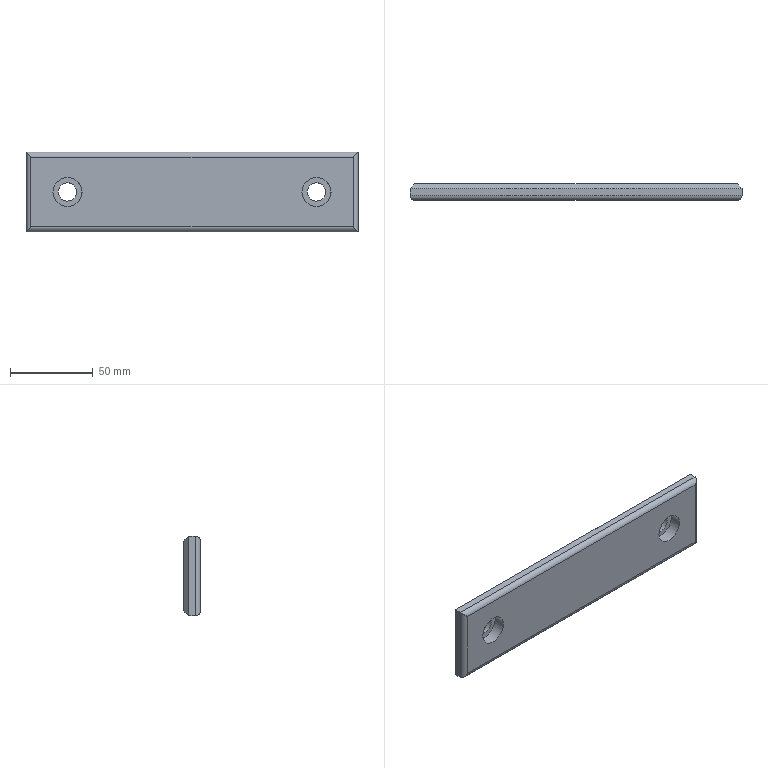Part | NX | features solid 2 | 1 solid | 20 faces | box 200 x 10 x 48 mm | volume 88919 mm3 | plane 12 | cylinder 8 | commonest cylinder face diameters 6 x4 11 x2 17.5 x2
STEP:
#1=CARTESIAN_POINT('',(85.,97.,-170.));
#2=VERTEX_POINT('',#1);
#3=CARTESIAN_POINT('',(85.,93.,-170.));
#4=VERTEX_POINT('',#3);
#5=CARTESIAN_POINT('',(85.,100.,-170.));
#6=DIRECTION('',(0.,-1.,0.));
#7=VECTOR('',#6,1000.);
#8=LINE('',#5,#7);
#9=EDGE_CURVE('',#2,#4,#8,.T.);
#10=ORIENTED_EDGE('',*,*,#9,.T.);
#11=CARTESIAN_POINT('',(85.,93.,-218.));
#12=VERTEX_POINT('',#11);
#13=CARTESIAN_POINT('',(85.,93.,-231.5));
#14=DIRECTION('',(0.,0.,1.));
#15=VECTOR('',#14,1000.);
#16=LINE('',#13,#15);
#17=EDGE_CURVE('',#12,#4,#16,.T.);
#18=ORIENTED_EDGE('',*,*,#17,.F.);
#19=CARTESIAN_POINT('',(85.,97.,-218.));
#20=VERTEX_POINT('',#19);
#21=CARTESIAN_POINT('',(85.,100.,-218.));
#22=DIRECTION('',(0.,-1.,0.));
#23=VECTOR('',#22,1000.);
#24=LINE('',#21,#23);
#25=EDGE_CURVE('',#20,#12,#24,.T.);
#26=ORIENTED_EDGE('',*,*,#25,.F.);
#27=CARTESIAN_POINT('',(85.,97.,-231.5));
#28=DIRECTION('',(0.,0.,-1.));
#29=VECTOR('',#28,1000.);
#30=LINE('',#27,#29);
#31=EDGE_CURVE('',#2,#20,#30,.T.);
#32=ORIENTED_EDGE('',*,*,#31,.F.);
#33=EDGE_LOOP('',(#10,#18,#26,#32));
#34=FACE_BOUND('',#33,.T.);
#35=CARTESIAN_POINT('',(85.,100.,-231.5));
#36=DIRECTION('',(-1.,0.,0.));
#37=DIRECTION('',(0.,-1.,0.));
#38=AXIS2_PLACEMENT_3D('',#35,#36,#37);
#39=PLANE('',#38);
#40=ADVANCED_FACE('',(#34),#39,.F.);
#41=CARTESIAN_POINT('',(-115.,97.,-170.));
#42=VERTEX_POINT('',#41);
#43=CARTESIAN_POINT('',(-115.,93.,-170.));
#44=VERTEX_POINT('',#43);
#45=CARTESIAN_POINT('',(-115.,100.,-170.));
#46=DIRECTION('',(0.,-1.,0.));
#47=VECTOR('',#46,1000.);
#48=LINE('',#45,#47);
#49=EDGE_CURVE('',#42,#44,#48,.T.);
#50=ORIENTED_EDGE('',*,*,#49,.T.);
#51=CARTESIAN_POINT('',(85.,93.,-170.));
#52=DIRECTION('',(-1.,0.,0.));
#53=VECTOR('',#52,1000.);
#54=LINE('',#51,#53);
#55=EDGE_CURVE('',#4,#44,#54,.T.);
#56=ORIENTED_EDGE('',*,*,#55,.F.);
#57=ORIENTED_EDGE('',*,*,#9,.F.);
#58=CARTESIAN_POINT('',(85.,97.,-170.));
#59=DIRECTION('',(1.,0.,0.));
#60=VECTOR('',#59,1000.);
#61=LINE('',#58,#60);
#62=EDGE_CURVE('',#42,#2,#61,.T.);
#63=ORIENTED_EDGE('',*,*,#62,.F.);
#64=EDGE_LOOP('',(#50,#56,#57,#63));
#65=FACE_BOUND('',#64,.T.);
#66=CARTESIAN_POINT('',(85.,100.,-170.));
#67=DIRECTION('',(0.,0.,-1.));
#68=DIRECTION('',(0.,1.,0.));
#69=AXIS2_PLACEMENT_3D('',#66,#67,#68);
#70=PLANE('',#69);
#71=ADVANCED_FACE('',(#65),#70,.F.);
#72=CARTESIAN_POINT('',(-115.,97.,-218.));
#73=VERTEX_POINT('',#72);
#74=CARTESIAN_POINT('',(-115.,93.,-218.));
#75=VERTEX_POINT('',#74);
#76=CARTESIAN_POINT('',(-115.,100.,-218.));
#77=DIRECTION('',(0.,-1.,0.));
#78=VECTOR('',#77,1000.);
#79=LINE('',#76,#78);
#80=EDGE_CURVE('',#73,#75,#79,.T.);
#81=ORIENTED_EDGE('',*,*,#80,.T.);
#82=CARTESIAN_POINT('',(-115.,93.,-156.5));
#83=DIRECTION('',(0.,0.,-1.));
#84=VECTOR('',#83,1000.);
#85=LINE('',#82,#84);
#86=EDGE_CURVE('',#44,#75,#85,.T.);
#87=ORIENTED_EDGE('',*,*,#86,.F.);
#88=ORIENTED_EDGE('',*,*,#49,.F.);
#89=CARTESIAN_POINT('',(-115.,97.,-156.5));
#90=DIRECTION('',(0.,0.,1.));
#91=VECTOR('',#90,1000.);
#92=LINE('',#89,#91);
#93=EDGE_CURVE('',#73,#42,#92,.T.);
#94=ORIENTED_EDGE('',*,*,#93,.F.);
#95=EDGE_LOOP('',(#81,#87,#88,#94));
#96=FACE_BOUND('',#95,.T.);
#97=CARTESIAN_POINT('',(-115.,100.,-156.5));
#98=DIRECTION('',(1.,0.,0.));
#99=DIRECTION('',(0.,1.,0.));
#100=AXIS2_PLACEMENT_3D('',#97,#98,#99);
#101=PLANE('',#100);
#102=ADVANCED_FACE('',(#96),#101,.F.);
#103=ORIENTED_EDGE('',*,*,#25,.T.);
#104=CARTESIAN_POINT('',(-115.,93.,-218.));
#105=DIRECTION('',(1.,0.,0.));
#106=VECTOR('',#105,1000.);
#107=LINE('',#104,#106);
#108=EDGE_CURVE('',#75,#12,#107,.T.);
#109=ORIENTED_EDGE('',*,*,#108,.F.);
#110=ORIENTED_EDGE('',*,*,#80,.F.);
#111=CARTESIAN_POINT('',(-115.,97.,-218.));
#112=DIRECTION('',(-1.,0.,0.));
#113=VECTOR('',#112,1000.);
#114=LINE('',#111,#113);
#115=EDGE_CURVE('',#20,#73,#114,.T.);
#116=ORIENTED_EDGE('',*,*,#115,.F.);
#117=EDGE_LOOP('',(#103,#109,#110,#116));
#118=FACE_BOUND('',#117,.T.);
#119=CARTESIAN_POINT('',(-115.,100.,-218.));
#120=DIRECTION('',(0.,0.,1.));
#121=DIRECTION('',(-1.,0.,0.));
#122=AXIS2_PLACEMENT_3D('',#119,#120,#121);
#123=PLANE('',#122);
#124=ADVANCED_FACE('',(#118),#123,.F.);
#125=CARTESIAN_POINT('',(82.,100.,-173.));
#126=VERTEX_POINT('',#125);
#127=CARTESIAN_POINT('',(-112.,100.,-173.));
#128=VERTEX_POINT('',#127);
#129=CARTESIAN_POINT('',(-115.,100.,-173.));
#130=DIRECTION('',(-1.,0.,0.));
#131=VECTOR('',#130,1000.);
#132=LINE('',#129,#131);
#133=EDGE_CURVE('',#126,#128,#132,.T.);
#134=ORIENTED_EDGE('',*,*,#133,.F.);
#135=CARTESIAN_POINT('',(82.,100.,-215.));
#136=VERTEX_POINT('',#135);
#137=CARTESIAN_POINT('',(82.,100.,-156.5));
#138=DIRECTION('',(0.,0.,1.));
#139=VECTOR('',#138,1000.);
#140=LINE('',#137,#139);
#141=EDGE_CURVE('',#136,#126,#140,.T.);
#142=ORIENTED_EDGE('',*,*,#141,.F.);
#143=CARTESIAN_POINT('',(-112.,100.,-215.));
#144=VERTEX_POINT('',#143);
#145=CARTESIAN_POINT('',(85.,100.,-215.));
#146=DIRECTION('',(1.,0.,0.));
#147=VECTOR('',#146,1000.);
#148=LINE('',#145,#147);
#149=EDGE_CURVE('',#144,#136,#148,.T.);
#150=ORIENTED_EDGE('',*,*,#149,.F.);
#151=CARTESIAN_POINT('',(-112.,100.,-231.5));
#152=DIRECTION('',(0.,0.,-1.));
#153=VECTOR('',#152,1000.);
#154=LINE('',#151,#153);
#155=EDGE_CURVE('',#128,#144,#154,.T.);
#156=ORIENTED_EDGE('',*,*,#155,.F.);
#157=EDGE_LOOP('',(#134,#142,#150,#156));
#158=FACE_BOUND('',#157,.T.);
#159=CARTESIAN_POINT('',(-95.5,100.,-194.));
#160=VERTEX_POINT('',#159);
#161=CARTESIAN_POINT('',(-90.,100.,-194.));
#162=DIRECTION('',(0.,-1.,0.));
#163=DIRECTION('',(-1.,0.,0.));
#164=AXIS2_PLACEMENT_3D('',#161,#162,#163);
#165=CIRCLE('',#164,5.5);
#166=EDGE_CURVE('',#160,#160,#165,.T.);
#167=ORIENTED_EDGE('',*,*,#166,.T.);
#168=EDGE_LOOP('',(#167));
#169=FACE_BOUND('',#168,.T.);
#170=CARTESIAN_POINT('',(54.5,100.,-194.));
#171=VERTEX_POINT('',#170);
#172=CARTESIAN_POINT('',(60.,100.,-194.));
#173=DIRECTION('',(0.,-1.,0.));
#174=DIRECTION('',(-1.,0.,0.));
#175=AXIS2_PLACEMENT_3D('',#172,#173,#174);
#176=CIRCLE('',#175,5.5);
#177=EDGE_CURVE('',#171,#171,#176,.T.);
#178=ORIENTED_EDGE('',*,*,#177,.T.);
#179=EDGE_LOOP('',(#178));
#180=FACE_BOUND('',#179,.T.);
#181=CARTESIAN_POINT('',(85.,100.,-156.5));
#182=DIRECTION('',(0.,1.,0.));
#183=DIRECTION('',(-1.,0.,0.));
#184=AXIS2_PLACEMENT_3D('',#181,#182,#183);
#185=PLANE('',#184);
#186=ADVANCED_FACE('',(#158,#169,#180),#185,.T.);
#187=CARTESIAN_POINT('',(82.,90.,-173.));
#188=VERTEX_POINT('',#187);
#189=CARTESIAN_POINT('',(82.,90.,-215.));
#190=VERTEX_POINT('',#189);
#191=CARTESIAN_POINT('',(82.,90.,-156.5));
#192=DIRECTION('',(0.,0.,1.));
#193=VECTOR('',#192,1000.);
#194=LINE('',#191,#193);
#195=EDGE_CURVE('',#188,#190,#194,.F.);
#196=ORIENTED_EDGE('',*,*,#195,.F.);
#197=CARTESIAN_POINT('',(-112.,90.,-173.));
#198=VERTEX_POINT('',#197);
#199=CARTESIAN_POINT('',(85.,90.,-173.));
#200=DIRECTION('',(-1.,0.,0.));
#201=VECTOR('',#200,1000.);
#202=LINE('',#199,#201);
#203=EDGE_CURVE('',#198,#188,#202,.F.);
#204=ORIENTED_EDGE('',*,*,#203,.F.);
#205=CARTESIAN_POINT('',(-112.,90.,-215.));
#206=VERTEX_POINT('',#205);
#207=CARTESIAN_POINT('',(-112.,90.,-156.5));
#208=DIRECTION('',(0.,0.,-1.));
#209=VECTOR('',#208,1000.);
#210=LINE('',#207,#209);
#211=EDGE_CURVE('',#206,#198,#210,.F.);
#212=ORIENTED_EDGE('',*,*,#211,.F.);
#213=CARTESIAN_POINT('',(85.,90.,-215.));
#214=DIRECTION('',(1.,0.,0.));
#215=VECTOR('',#214,1000.);
#216=LINE('',#213,#215);
#217=EDGE_CURVE('',#190,#206,#216,.F.);
#218=ORIENTED_EDGE('',*,*,#217,.F.);
#219=EDGE_LOOP('',(#196,#204,#212,#218));
#220=FACE_BOUND('',#219,.T.);
#221=CARTESIAN_POINT('',(-98.75,90.,-194.));
#222=VERTEX_POINT('',#221);
#223=CARTESIAN_POINT('',(-90.,90.,-194.));
#224=DIRECTION('',(0.,-1.,0.));
#225=DIRECTION('',(-1.,0.,0.));
#226=AXIS2_PLACEMENT_3D('',#223,#224,#225);
#227=CIRCLE('',#226,8.75);
#228=EDGE_CURVE('',#222,#222,#227,.T.);
#229=ORIENTED_EDGE('',*,*,#228,.F.);
#230=EDGE_LOOP('',(#229));
#231=FACE_BOUND('',#230,.T.);
#232=CARTESIAN_POINT('',(51.25,90.,-194.));
#233=VERTEX_POINT('',#232);
#234=CARTESIAN_POINT('',(60.,90.,-194.));
#235=DIRECTION('',(0.,-1.,0.));
#236=DIRECTION('',(-1.,0.,0.));
#237=AXIS2_PLACEMENT_3D('',#234,#235,#236);
#238=CIRCLE('',#237,8.75);
#239=EDGE_CURVE('',#233,#233,#238,.T.);
#240=ORIENTED_EDGE('',*,*,#239,.F.);
#241=EDGE_LOOP('',(#240));
#242=FACE_BOUND('',#241,.T.);
#243=CARTESIAN_POINT('',(85.,90.,-156.5));
#244=DIRECTION('',(0.,1.,0.));
#245=DIRECTION('',(-1.,0.,0.));
#246=AXIS2_PLACEMENT_3D('',#243,#244,#245);
#247=PLANE('',#246);
#248=ADVANCED_FACE('',(#220,#231,#242),#247,.F.);
#249=ORIENTED_EDGE('',*,*,#177,.F.);
#250=EDGE_LOOP('',(#249));
#251=FACE_BOUND('',#250,.T.);
#252=CARTESIAN_POINT('',(60.,97.,-199.5));
#253=VERTEX_POINT('',#252);
#254=CARTESIAN_POINT('',(60.,97.,-194.));
#255=DIRECTION('',(0.,-1.,0.));
#256=DIRECTION('',(0.,0.,-1.));
#257=AXIS2_PLACEMENT_3D('',#254,#255,#256);
#258=CIRCLE('',#257,5.5);
#259=EDGE_CURVE('',#253,#253,#258,.T.);
#260=ORIENTED_EDGE('',*,*,#259,.T.);
#261=EDGE_LOOP('',(#260));
#262=FACE_BOUND('',#261,.T.);
#263=CARTESIAN_POINT('',(60.,130.,-194.));
#264=DIRECTION('',(0.,1.,0.));
#265=DIRECTION('',(-1.,0.,0.));
#266=AXIS2_PLACEMENT_3D('',#263,#264,#265);
#267=CYLINDRICAL_SURFACE('',#266,5.5);
#268=ADVANCED_FACE('',(#251,#262),#267,.F.);
#269=ORIENTED_EDGE('',*,*,#259,.F.);
#270=EDGE_LOOP('',(#269));
#271=FACE_BOUND('',#270,.T.);
#272=CARTESIAN_POINT('',(60.,97.,-202.75));
#273=VERTEX_POINT('',#272);
#274=CARTESIAN_POINT('',(60.,97.,-194.));
#275=DIRECTION('',(0.,-1.,0.));
#276=DIRECTION('',(0.,0.,-1.));
#277=AXIS2_PLACEMENT_3D('',#274,#275,#276);
#278=CIRCLE('',#277,8.75);
#279=EDGE_CURVE('',#273,#273,#278,.T.);
#280=ORIENTED_EDGE('',*,*,#279,.T.);
#281=EDGE_LOOP('',(#280));
#282=FACE_BOUND('',#281,.T.);
#283=CARTESIAN_POINT('',(60.,97.,-194.));
#284=DIRECTION('',(0.,1.,0.));
#285=DIRECTION('',(-1.,0.,0.));
#286=AXIS2_PLACEMENT_3D('',#283,#284,#285);
#287=PLANE('',#286);
#288=ADVANCED_FACE('',(#271,#282),#287,.F.);
#289=ORIENTED_EDGE('',*,*,#279,.F.);
#290=EDGE_LOOP('',(#289));
#291=FACE_BOUND('',#290,.T.);
#292=ORIENTED_EDGE('',*,*,#239,.T.);
#293=EDGE_LOOP('',(#292));
#294=FACE_BOUND('',#293,.T.);
#295=CARTESIAN_POINT('',(60.,80.,-194.));
#296=DIRECTION('',(0.,1.,0.));
#297=DIRECTION('',(-1.,0.,0.));
#298=AXIS2_PLACEMENT_3D('',#295,#296,#297);
#299=CYLINDRICAL_SURFACE('',#298,8.75);
#300=ADVANCED_FACE('',(#291,#294),#299,.F.);
#301=ORIENTED_EDGE('',*,*,#166,.F.);
#302=EDGE_LOOP('',(#301));
#303=FACE_BOUND('',#302,.T.);
#304=CARTESIAN_POINT('',(-90.,97.,-199.5));
#305=VERTEX_POINT('',#304);
#306=CARTESIAN_POINT('',(-90.,97.,-194.));
#307=DIRECTION('',(0.,-1.,0.));
#308=DIRECTION('',(0.,0.,-1.));
#309=AXIS2_PLACEMENT_3D('',#306,#307,#308);
#310=CIRCLE('',#309,5.5);
#311=EDGE_CURVE('',#305,#305,#310,.T.);
#312=ORIENTED_EDGE('',*,*,#311,.T.);
#313=EDGE_LOOP('',(#312));
#314=FACE_BOUND('',#313,.T.);
#315=CARTESIAN_POINT('',(-90.,130.,-194.));
#316=DIRECTION('',(0.,1.,0.));
#317=DIRECTION('',(-1.,0.,0.));
#318=AXIS2_PLACEMENT_3D('',#315,#316,#317);
#319=CYLINDRICAL_SURFACE('',#318,5.5);
#320=ADVANCED_FACE('',(#303,#314),#319,.F.);
#321=ORIENTED_EDGE('',*,*,#311,.F.);
#322=EDGE_LOOP('',(#321));
#323=FACE_BOUND('',#322,.T.);
#324=CARTESIAN_POINT('',(-90.,97.,-202.75));
#325=VERTEX_POINT('',#324);
#326=CARTESIAN_POINT('',(-90.,97.,-194.));
#327=DIRECTION('',(0.,-1.,0.));
#328=DIRECTION('',(0.,0.,-1.));
#329=AXIS2_PLACEMENT_3D('',#326,#327,#328);
#330=CIRCLE('',#329,8.75);
#331=EDGE_CURVE('',#325,#325,#330,.T.);
#332=ORIENTED_EDGE('',*,*,#331,.T.);
#333=EDGE_LOOP('',(#332));
#334=FACE_BOUND('',#333,.T.);
#335=CARTESIAN_POINT('',(-90.,97.,-194.));
#336=DIRECTION('',(0.,1.,0.));
#337=DIRECTION('',(-1.,0.,0.));
#338=AXIS2_PLACEMENT_3D('',#335,#336,#337);
#339=PLANE('',#338);
#340=ADVANCED_FACE('',(#323,#334),#339,.F.);
#341=ORIENTED_EDGE('',*,*,#331,.F.);
#342=EDGE_LOOP('',(#341));
#343=FACE_BOUND('',#342,.T.);
#344=ORIENTED_EDGE('',*,*,#228,.T.);
#345=EDGE_LOOP('',(#344));
#346=FACE_BOUND('',#345,.T.);
#347=CARTESIAN_POINT('',(-90.,80.,-194.));
#348=DIRECTION('',(0.,1.,0.));
#349=DIRECTION('',(-1.,0.,0.));
#350=AXIS2_PLACEMENT_3D('',#347,#348,#349);
#351=CYLINDRICAL_SURFACE('',#350,8.75);
#352=ADVANCED_FACE('',(#343,#346),#351,.F.);
#353=CARTESIAN_POINT('',(82.,93.,-173.));
#354=DIRECTION('',(0.7071,0.,-0.7071));
#355=DIRECTION('',(0.7071,0.,0.7071));
#356=AXIS2_PLACEMENT_3D('',#353,#354,#355);
#357=ELLIPSE('',#356,4.243,3.);
#358=EDGE_CURVE('',#188,#4,#357,.F.);
#359=ORIENTED_EDGE('',*,*,#358,.T.);
#360=ORIENTED_EDGE('',*,*,#55,.T.);
#361=CARTESIAN_POINT('',(-112.,93.,-173.));
#362=DIRECTION('',(0.7071,0.,0.7071));
#363=DIRECTION('',(-0.7071,0.,0.7071));
#364=AXIS2_PLACEMENT_3D('',#361,#362,#363);
#365=ELLIPSE('',#364,4.243,3.);
#366=EDGE_CURVE('',#44,#198,#365,.T.);
#367=ORIENTED_EDGE('',*,*,#366,.T.);
#368=ORIENTED_EDGE('',*,*,#203,.T.);
#369=EDGE_LOOP('',(#359,#360,#367,#368));
#370=FACE_BOUND('',#369,.T.);
#371=CARTESIAN_POINT('',(85.,93.,-173.));
#372=DIRECTION('',(-1.,0.,0.));
#373=DIRECTION('',(0.,-1.,0.));
#374=AXIS2_PLACEMENT_3D('',#371,#372,#373);
#375=CYLINDRICAL_SURFACE('',#374,3.);
#376=ADVANCED_FACE('',(#370),#375,.T.);
#377=ORIENTED_EDGE('',*,*,#366,.F.);
#378=ORIENTED_EDGE('',*,*,#86,.T.);
#379=CARTESIAN_POINT('',(-112.,93.,-215.));
#380=DIRECTION('',(-0.7071,0.,0.7071));
#381=DIRECTION('',(-0.7071,0.,-0.7071));
#382=AXIS2_PLACEMENT_3D('',#379,#380,#381);
#383=ELLIPSE('',#382,4.243,3.);
#384=EDGE_CURVE('',#75,#206,#383,.T.);
#385=ORIENTED_EDGE('',*,*,#384,.T.);
#386=ORIENTED_EDGE('',*,*,#211,.T.);
#387=EDGE_LOOP('',(#377,#378,#385,#386));
#388=FACE_BOUND('',#387,.T.);
#389=CARTESIAN_POINT('',(-112.,93.,-156.5));
#390=DIRECTION('',(0.,0.,-1.));
#391=DIRECTION('',(0.,1.,0.));
#392=AXIS2_PLACEMENT_3D('',#389,#390,#391);
#393=CYLINDRICAL_SURFACE('',#392,3.);
#394=ADVANCED_FACE('',(#388),#393,.T.);
#395=ORIENTED_EDGE('',*,*,#358,.F.);
#396=ORIENTED_EDGE('',*,*,#195,.T.);
#397=CARTESIAN_POINT('',(82.,93.,-215.));
#398=DIRECTION('',(-0.7071,0.,-0.7071));
#399=DIRECTION('',(-0.7071,0.,0.7071));
#400=AXIS2_PLACEMENT_3D('',#397,#398,#399);
#401=ELLIPSE('',#400,4.243,3.);
#402=EDGE_CURVE('',#190,#12,#401,.F.);
#403=ORIENTED_EDGE('',*,*,#402,.T.);
#404=ORIENTED_EDGE('',*,*,#17,.T.);
#405=EDGE_LOOP('',(#395,#396,#403,#404));
#406=FACE_BOUND('',#405,.T.);
#407=CARTESIAN_POINT('',(82.,93.,-231.5));
#408=DIRECTION('',(0.,0.,1.));
#409=DIRECTION('',(0.,-1.,0.));
#410=AXIS2_PLACEMENT_3D('',#407,#408,#409);
#411=CYLINDRICAL_SURFACE('',#410,3.);
#412=ADVANCED_FACE('',(#406),#411,.T.);
#413=ORIENTED_EDGE('',*,*,#384,.F.);
#414=ORIENTED_EDGE('',*,*,#108,.T.);
#415=ORIENTED_EDGE('',*,*,#402,.F.);
#416=ORIENTED_EDGE('',*,*,#217,.T.);
#417=EDGE_LOOP('',(#413,#414,#415,#416));
#418=FACE_BOUND('',#417,.T.);
#419=CARTESIAN_POINT('',(-115.,93.,-215.));
#420=DIRECTION('',(1.,0.,0.));
#421=DIRECTION('',(0.,0.,1.));
#422=AXIS2_PLACEMENT_3D('',#419,#420,#421);
#423=CYLINDRICAL_SURFACE('',#422,3.);
#424=ADVANCED_FACE('',(#418),#423,.T.);
#425=CARTESIAN_POINT('',(83.,99.,-216.));
#426=DIRECTION('',(-0.5774,0.5774,0.5774));
#427=VECTOR('',#426,1000.);
#428=LINE('',#425,#427);
#429=EDGE_CURVE('',#20,#136,#428,.T.);
#430=ORIENTED_EDGE('',*,*,#429,.T.);
#431=ORIENTED_EDGE('',*,*,#141,.T.);
#432=CARTESIAN_POINT('',(83.,99.,-172.));
#433=DIRECTION('',(-0.5774,0.5774,-0.5774));
#434=VECTOR('',#433,1000.);
#435=LINE('',#432,#434);
#436=EDGE_CURVE('',#126,#2,#435,.F.);
#437=ORIENTED_EDGE('',*,*,#436,.T.);
#438=ORIENTED_EDGE('',*,*,#31,.T.);
#439=EDGE_LOOP('',(#430,#431,#437,#438));
#440=FACE_BOUND('',#439,.T.);
#441=CARTESIAN_POINT('',(82.,100.,-156.5));
#442=DIRECTION('',(0.7071,0.7071,0.));
#443=DIRECTION('',(-0.7071,0.7071,0.));
#444=AXIS2_PLACEMENT_3D('',#441,#442,#443);
#445=PLANE('',#444);
#446=ADVANCED_FACE('',(#440),#445,.T.);
#447=ORIENTED_EDGE('',*,*,#436,.F.);
#448=ORIENTED_EDGE('',*,*,#133,.T.);
#449=CARTESIAN_POINT('',(-46.333,165.667,-238.667));
#450=DIRECTION('',(0.5774,0.5774,-0.5774));
#451=VECTOR('',#450,1000.);
#452=LINE('',#449,#451);
#453=EDGE_CURVE('',#128,#42,#452,.F.);
#454=ORIENTED_EDGE('',*,*,#453,.T.);
#455=ORIENTED_EDGE('',*,*,#62,.T.);
#456=EDGE_LOOP('',(#447,#448,#454,#455));
#457=FACE_BOUND('',#456,.T.);
#458=CARTESIAN_POINT('',(85.,100.,-173.));
#459=DIRECTION('',(0.,0.7071,0.7071));
#460=DIRECTION('',(0.,-0.7071,0.7071));
#461=AXIS2_PLACEMENT_3D('',#458,#459,#460);
#462=PLANE('',#461);
#463=ADVANCED_FACE('',(#457),#462,.T.);
#464=ORIENTED_EDGE('',*,*,#429,.F.);
#465=ORIENTED_EDGE('',*,*,#115,.T.);
#466=CARTESIAN_POINT('',(-46.333,165.667,-149.333));
#467=DIRECTION('',(-0.5774,-0.5774,-0.5774));
#468=VECTOR('',#467,1000.);
#469=LINE('',#466,#468);
#470=EDGE_CURVE('',#73,#144,#469,.F.);
#471=ORIENTED_EDGE('',*,*,#470,.T.);
#472=ORIENTED_EDGE('',*,*,#149,.T.);
#473=EDGE_LOOP('',(#464,#465,#471,#472));
#474=FACE_BOUND('',#473,.T.);
#475=CARTESIAN_POINT('',(85.,100.,-215.));
#476=DIRECTION('',(0.,0.7071,-0.7071));
#477=DIRECTION('',(0.,0.7071,0.7071));
#478=AXIS2_PLACEMENT_3D('',#475,#476,#477);
#479=PLANE('',#478);
#480=ADVANCED_FACE('',(#474),#479,.T.);
#481=ORIENTED_EDGE('',*,*,#453,.F.);
#482=ORIENTED_EDGE('',*,*,#155,.T.);
#483=ORIENTED_EDGE('',*,*,#470,.F.);
#484=ORIENTED_EDGE('',*,*,#93,.T.);
#485=EDGE_LOOP('',(#481,#482,#483,#484));
#486=FACE_BOUND('',#485,.T.);
#487=CARTESIAN_POINT('',(-112.,100.,-156.5));
#488=DIRECTION('',(-0.7071,0.7071,0.));
#489=DIRECTION('',(-0.7071,-0.7071,0.));
#490=AXIS2_PLACEMENT_3D('',#487,#488,#489);
#491=PLANE('',#490);
#492=ADVANCED_FACE('',(#486),#491,.T.);
#493=CLOSED_SHELL('',(#40,#71,#102,#124,#186,#248,#268,#288,#300,#320,#340,#352,#376,#394,#412,#424,#446,#463,#480,#492));
#494=MANIFOLD_SOLID_BREP('',#493);
#495=(LENGTH_UNIT()NAMED_UNIT(*)SI_UNIT(.MILLI.,.METRE.));
#496=UNCERTAINTY_MEASURE_WITH_UNIT(LENGTH_MEASURE(0.00001),#495,'','');
#497=(NAMED_UNIT(*)PLANE_ANGLE_UNIT()SI_UNIT($,.RADIAN.));
#498=(NAMED_UNIT(*)SI_UNIT($,.STERADIAN.)SOLID_ANGLE_UNIT());
#499=(GEOMETRIC_REPRESENTATION_CONTEXT(3)GLOBAL_UNCERTAINTY_ASSIGNED_CONTEXT((#496))GLOBAL_UNIT_ASSIGNED_CONTEXT((#495,#497,#498))REPRESENTATION_CONTEXT('',''));
#500=ADVANCED_BREP_SHAPE_REPRESENTATION('',(#494),#499);